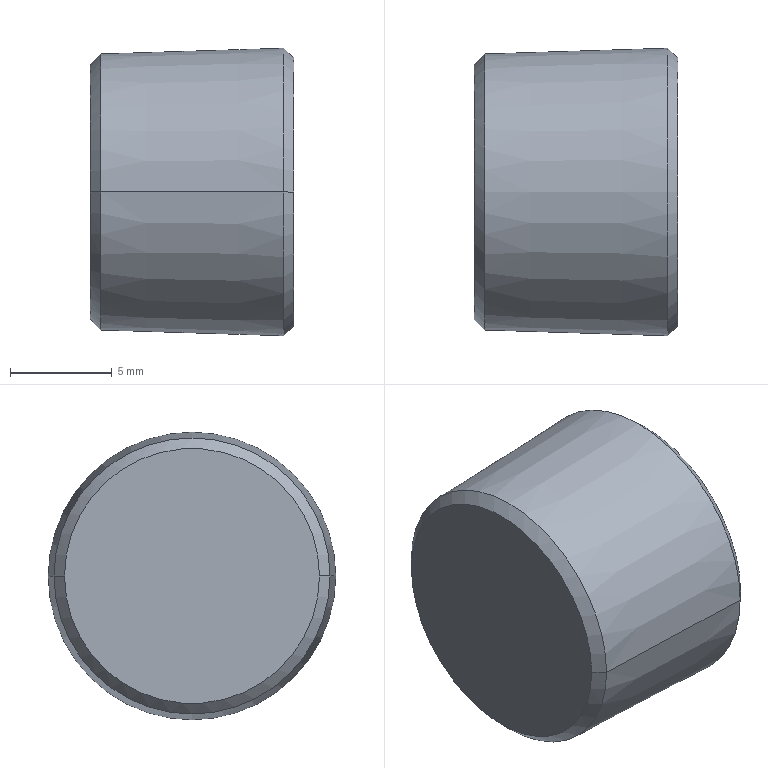Part | SolidWorks | features Chamfer 1, Cut 1, Revolution 1 | 1 solid | 15 faces | box 10 x 14.097 x 14.097 mm | volume 1197 mm3 | plane 9 | cone 6
STEP:
#1=CARTESIAN_POINT('',(0.,-6.25,0.));
#2=VERTEX_POINT('',#1);
#3=CARTESIAN_POINT('',(0.,6.25,0.));
#4=VERTEX_POINT('',#3);
#5=CARTESIAN_POINT('',(0.,0.,0.));
#6=DIRECTION('',(-1.,0.,0.));
#7=DIRECTION('',(0.,-1.,0.));
#8=AXIS2_PLACEMENT_3D('',#5,#6,#7);
#9=CIRCLE('',#8,6.25);
#10=EDGE_CURVE('',#2,#4,#9,.T.);
#11=ORIENTED_EDGE('',*,*,#10,.F.);
#12=CARTESIAN_POINT('',(0.5162,-6.766,0.));
#13=VERTEX_POINT('',#12);
#14=CARTESIAN_POINT('',(0.5162,-6.766,0.));
#15=DIRECTION('',(0.7071,-0.7071,0.));
#16=VECTOR('',#15,1000.);
#17=LINE('',#14,#16);
#18=EDGE_CURVE('',#2,#13,#17,.T.);
#19=ORIENTED_EDGE('',*,*,#18,.T.);
#20=CARTESIAN_POINT('',(0.5162,6.766,0.));
#21=VERTEX_POINT('',#20);
#22=CARTESIAN_POINT('',(0.5162,0.,0.));
#23=DIRECTION('',(1.,0.,0.));
#24=DIRECTION('',(0.,-1.,0.));
#25=AXIS2_PLACEMENT_3D('',#22,#23,#24);
#26=CIRCLE('',#25,6.766);
#27=EDGE_CURVE('',#21,#13,#26,.T.);
#28=ORIENTED_EDGE('',*,*,#27,.F.);
#29=CARTESIAN_POINT('',(0.5162,6.766,0.));
#30=DIRECTION('',(0.7071,0.7071,0.));
#31=VECTOR('',#30,1000.);
#32=LINE('',#29,#31);
#33=EDGE_CURVE('',#4,#21,#32,.T.);
#34=ORIENTED_EDGE('',*,*,#33,.F.);
#35=EDGE_LOOP('',(#11,#19,#28,#34));
#36=FACE_OUTER_BOUND('',#35,.T.);
#37=CARTESIAN_POINT('',(0.5162,0.,0.));
#38=DIRECTION('',(1.,0.,0.));
#39=DIRECTION('',(0.,1.,0.));
#40=AXIS2_PLACEMENT_3D('',#37,#38,#39);
#41=CONICAL_SURFACE('',#40,6.766,0.7854);
#42=ADVANCED_FACE('',(#36),#41,.T.);
#43=CARTESIAN_POINT('',(10.,6.579,0.));
#44=VERTEX_POINT('',#43);
#45=CARTESIAN_POINT('',(10.,-6.579,0.));
#46=VERTEX_POINT('',#45);
#47=CARTESIAN_POINT('',(10.,0.,0.));
#48=DIRECTION('',(1.,0.,0.));
#49=DIRECTION('',(0.,1.,0.));
#50=AXIS2_PLACEMENT_3D('',#47,#48,#49);
#51=CIRCLE('',#50,6.579);
#52=EDGE_CURVE('',#44,#46,#51,.T.);
#53=ORIENTED_EDGE('',*,*,#52,.F.);
#54=CARTESIAN_POINT('',(9.5,7.049,0.));
#55=VERTEX_POINT('',#54);
#56=CARTESIAN_POINT('',(10.,6.579,0.));
#57=DIRECTION('',(-0.729,0.6845,0.));
#58=VECTOR('',#57,1000.);
#59=LINE('',#56,#58);
#60=EDGE_CURVE('',#44,#55,#59,.T.);
#61=ORIENTED_EDGE('',*,*,#60,.T.);
#62=CARTESIAN_POINT('',(9.5,-7.049,0.));
#63=VERTEX_POINT('',#62);
#64=CARTESIAN_POINT('',(9.5,0.,0.));
#65=DIRECTION('',(-1.,0.,0.));
#66=DIRECTION('',(0.,-1.,0.));
#67=AXIS2_PLACEMENT_3D('',#64,#65,#66);
#68=CIRCLE('',#67,7.049);
#69=EDGE_CURVE('',#63,#55,#68,.T.);
#70=ORIENTED_EDGE('',*,*,#69,.F.);
#71=CARTESIAN_POINT('',(10.,-6.579,0.));
#72=DIRECTION('',(-0.729,-0.6845,0.));
#73=VECTOR('',#72,1000.);
#74=LINE('',#71,#73);
#75=EDGE_CURVE('',#46,#63,#74,.T.);
#76=ORIENTED_EDGE('',*,*,#75,.F.);
#77=EDGE_LOOP('',(#53,#61,#70,#76));
#78=FACE_OUTER_BOUND('',#77,.T.);
#79=CARTESIAN_POINT('',(10.,0.,0.));
#80=DIRECTION('',(-1.,0.,0.));
#81=DIRECTION('',(0.,-1.,0.));
#82=AXIS2_PLACEMENT_3D('',#79,#80,#81);
#83=CONICAL_SURFACE('',#82,6.579,0.754);
#84=ADVANCED_FACE('',(#78),#83,.T.);
#85=ORIENTED_EDGE('',*,*,#27,.T.);
#86=CARTESIAN_POINT('',(10.,-7.064,0.));
#87=DIRECTION('',(0.9995,-0.03141,0.));
#88=VECTOR('',#87,1000.);
#89=LINE('',#86,#88);
#90=EDGE_CURVE('',#13,#63,#89,.T.);
#91=ORIENTED_EDGE('',*,*,#90,.T.);
#92=ORIENTED_EDGE('',*,*,#69,.T.);
#93=CARTESIAN_POINT('',(10.,7.064,0.));
#94=DIRECTION('',(0.9995,0.03141,0.));
#95=VECTOR('',#94,1000.);
#96=LINE('',#93,#95);
#97=EDGE_CURVE('',#21,#55,#96,.T.);
#98=ORIENTED_EDGE('',*,*,#97,.F.);
#99=EDGE_LOOP('',(#85,#91,#92,#98));
#100=FACE_OUTER_BOUND('',#99,.T.);
#101=CARTESIAN_POINT('',(10.,0.,0.));
#102=DIRECTION('',(1.,0.,0.));
#103=DIRECTION('',(0.,1.,0.));
#104=AXIS2_PLACEMENT_3D('',#101,#102,#103);
#105=CONICAL_SURFACE('',#104,7.064,0.03142);
#106=ADVANCED_FACE('',(#100),#105,.T.);
#107=CARTESIAN_POINT('',(10.,0.,0.));
#108=DIRECTION('',(1.,0.,0.));
#109=DIRECTION('',(0.,1.,0.));
#110=AXIS2_PLACEMENT_3D('',#107,#108,#109);
#111=CIRCLE('',#110,6.579);
#112=EDGE_CURVE('',#46,#44,#111,.T.);
#113=ORIENTED_EDGE('',*,*,#112,.T.);
#114=ORIENTED_EDGE('',*,*,#52,.T.);
#115=EDGE_LOOP('',(#113,#114));
#116=FACE_OUTER_BOUND('',#115,.T.);
#117=CARTESIAN_POINT('',(10.,-4.1,2.367));
#118=VERTEX_POINT('',#117);
#119=CARTESIAN_POINT('',(10.,-4.1,-2.367));
#120=VERTEX_POINT('',#119);
#121=CARTESIAN_POINT('',(10.,-4.1,2.367));
#122=DIRECTION('',(0.,0.,-1.));
#123=VECTOR('',#122,1000.);
#124=LINE('',#121,#123);
#125=EDGE_CURVE('',#118,#120,#124,.T.);
#126=ORIENTED_EDGE('',*,*,#125,.F.);
#127=CARTESIAN_POINT('',(10.,0.,4.734));
#128=VERTEX_POINT('',#127);
#129=CARTESIAN_POINT('',(10.,0.,4.734));
#130=DIRECTION('',(0.,-0.866,-0.5));
#131=VECTOR('',#130,1000.);
#132=LINE('',#129,#131);
#133=EDGE_CURVE('',#128,#118,#132,.T.);
#134=ORIENTED_EDGE('',*,*,#133,.F.);
#135=CARTESIAN_POINT('',(10.,4.1,2.367));
#136=VERTEX_POINT('',#135);
#137=CARTESIAN_POINT('',(10.,4.1,2.367));
#138=DIRECTION('',(0.,-0.866,0.5));
#139=VECTOR('',#138,1000.);
#140=LINE('',#137,#139);
#141=EDGE_CURVE('',#136,#128,#140,.T.);
#142=ORIENTED_EDGE('',*,*,#141,.F.);
#143=CARTESIAN_POINT('',(10.,4.1,-2.367));
#144=VERTEX_POINT('',#143);
#145=CARTESIAN_POINT('',(10.,4.1,-2.367));
#146=DIRECTION('',(0.,0.,1.));
#147=VECTOR('',#146,1000.);
#148=LINE('',#145,#147);
#149=EDGE_CURVE('',#144,#136,#148,.T.);
#150=ORIENTED_EDGE('',*,*,#149,.F.);
#151=CARTESIAN_POINT('',(10.,0.,-4.734));
#152=VERTEX_POINT('',#151);
#153=CARTESIAN_POINT('',(10.,0.,-4.734));
#154=DIRECTION('',(0.,0.866,0.5));
#155=VECTOR('',#154,1000.);
#156=LINE('',#153,#155);
#157=EDGE_CURVE('',#152,#144,#156,.T.);
#158=ORIENTED_EDGE('',*,*,#157,.F.);
#159=CARTESIAN_POINT('',(10.,-4.1,-2.367));
#160=DIRECTION('',(0.,0.866,-0.5));
#161=VECTOR('',#160,1000.);
#162=LINE('',#159,#161);
#163=EDGE_CURVE('',#120,#152,#162,.T.);
#164=ORIENTED_EDGE('',*,*,#163,.F.);
#165=EDGE_LOOP('',(#126,#134,#142,#150,#158,#164));
#166=FACE_BOUND('',#165,.T.);
#167=CARTESIAN_POINT('',(10.,7.064,0.));
#168=DIRECTION('',(1.,0.,0.));
#169=DIRECTION('',(0.,1.,0.));
#170=AXIS2_PLACEMENT_3D('',#167,#168,#169);
#171=PLANE('',#170);
#172=ADVANCED_FACE('',(#116,#166),#171,.T.);
#173=ORIENTED_EDGE('',*,*,#90,.F.);
#174=CARTESIAN_POINT('',(0.5162,0.,0.));
#175=DIRECTION('',(1.,0.,0.));
#176=DIRECTION('',(0.,-1.,0.));
#177=AXIS2_PLACEMENT_3D('',#174,#175,#176);
#178=CIRCLE('',#177,6.766);
#179=EDGE_CURVE('',#13,#21,#178,.T.);
#180=ORIENTED_EDGE('',*,*,#179,.T.);
#181=ORIENTED_EDGE('',*,*,#97,.T.);
#182=CARTESIAN_POINT('',(9.5,0.,0.));
#183=DIRECTION('',(-1.,0.,0.));
#184=DIRECTION('',(0.,-1.,0.));
#185=AXIS2_PLACEMENT_3D('',#182,#183,#184);
#186=CIRCLE('',#185,7.049);
#187=EDGE_CURVE('',#55,#63,#186,.T.);
#188=ORIENTED_EDGE('',*,*,#187,.T.);
#189=EDGE_LOOP('',(#173,#180,#181,#188));
#190=FACE_OUTER_BOUND('',#189,.T.);
#191=CARTESIAN_POINT('',(10.,0.,0.));
#192=DIRECTION('',(1.,0.,0.));
#193=DIRECTION('',(0.,1.,0.));
#194=AXIS2_PLACEMENT_3D('',#191,#192,#193);
#195=CONICAL_SURFACE('',#194,7.064,0.03142);
#196=ADVANCED_FACE('',(#190),#195,.T.);
#197=CARTESIAN_POINT('',(0.,0.,0.));
#198=DIRECTION('',(-1.,0.,0.));
#199=DIRECTION('',(0.,-1.,0.));
#200=AXIS2_PLACEMENT_3D('',#197,#198,#199);
#201=CIRCLE('',#200,6.25);
#202=EDGE_CURVE('',#4,#2,#201,.T.);
#203=ORIENTED_EDGE('',*,*,#202,.T.);
#204=ORIENTED_EDGE('',*,*,#10,.T.);
#205=EDGE_LOOP('',(#203,#204));
#206=FACE_OUTER_BOUND('',#205,.T.);
#207=CARTESIAN_POINT('',(0.,0.,0.));
#208=DIRECTION('',(-1.,0.,0.));
#209=DIRECTION('',(0.,-1.,0.));
#210=AXIS2_PLACEMENT_3D('',#207,#208,#209);
#211=PLANE('',#210);
#212=ADVANCED_FACE('',(#206),#211,.T.);
#213=ORIENTED_EDGE('',*,*,#125,.T.);
#214=CARTESIAN_POINT('',(5.,-4.1,-2.367));
#215=VERTEX_POINT('',#214);
#216=CARTESIAN_POINT('',(5.,-4.1,-2.367));
#217=DIRECTION('',(1.,0.,0.));
#218=VECTOR('',#217,1000.);
#219=LINE('',#216,#218);
#220=EDGE_CURVE('',#215,#120,#219,.T.);
#221=ORIENTED_EDGE('',*,*,#220,.F.);
#222=CARTESIAN_POINT('',(5.,-4.1,2.367));
#223=VERTEX_POINT('',#222);
#224=CARTESIAN_POINT('',(5.,-4.1,2.367));
#225=DIRECTION('',(0.,0.,-1.));
#226=VECTOR('',#225,1000.);
#227=LINE('',#224,#226);
#228=EDGE_CURVE('',#223,#215,#227,.T.);
#229=ORIENTED_EDGE('',*,*,#228,.F.);
#230=CARTESIAN_POINT('',(5.,-4.1,2.367));
#231=DIRECTION('',(1.,0.,0.));
#232=VECTOR('',#231,1000.);
#233=LINE('',#230,#232);
#234=EDGE_CURVE('',#223,#118,#233,.T.);
#235=ORIENTED_EDGE('',*,*,#234,.T.);
#236=EDGE_LOOP('',(#213,#221,#229,#235));
#237=FACE_OUTER_BOUND('',#236,.T.);
#238=CARTESIAN_POINT('',(5.,-4.1,2.367));
#239=DIRECTION('',(0.,-1.,0.));
#240=DIRECTION('',(0.,0.,-1.));
#241=AXIS2_PLACEMENT_3D('',#238,#239,#240);
#242=PLANE('',#241);
#243=ADVANCED_FACE('',(#237),#242,.F.);
#244=ORIENTED_EDGE('',*,*,#133,.T.);
#245=ORIENTED_EDGE('',*,*,#234,.F.);
#246=CARTESIAN_POINT('',(5.,0.,4.734));
#247=VERTEX_POINT('',#246);
#248=CARTESIAN_POINT('',(5.,0.,4.734));
#249=DIRECTION('',(0.,-0.866,-0.5));
#250=VECTOR('',#249,1000.);
#251=LINE('',#248,#250);
#252=EDGE_CURVE('',#247,#223,#251,.T.);
#253=ORIENTED_EDGE('',*,*,#252,.F.);
#254=CARTESIAN_POINT('',(5.,0.,4.734));
#255=DIRECTION('',(1.,0.,0.));
#256=VECTOR('',#255,1000.);
#257=LINE('',#254,#256);
#258=EDGE_CURVE('',#247,#128,#257,.T.);
#259=ORIENTED_EDGE('',*,*,#258,.T.);
#260=EDGE_LOOP('',(#244,#245,#253,#259));
#261=FACE_OUTER_BOUND('',#260,.T.);
#262=CARTESIAN_POINT('',(5.,0.,4.734));
#263=DIRECTION('',(0.,-0.5,0.866));
#264=DIRECTION('',(0.,-0.866,-0.5));
#265=AXIS2_PLACEMENT_3D('',#262,#263,#264);
#266=PLANE('',#265);
#267=ADVANCED_FACE('',(#261),#266,.F.);
#268=ORIENTED_EDGE('',*,*,#141,.T.);
#269=ORIENTED_EDGE('',*,*,#258,.F.);
#270=CARTESIAN_POINT('',(5.,4.1,2.367));
#271=VERTEX_POINT('',#270);
#272=CARTESIAN_POINT('',(5.,4.1,2.367));
#273=DIRECTION('',(0.,-0.866,0.5));
#274=VECTOR('',#273,1000.);
#275=LINE('',#272,#274);
#276=EDGE_CURVE('',#271,#247,#275,.T.);
#277=ORIENTED_EDGE('',*,*,#276,.F.);
#278=CARTESIAN_POINT('',(5.,4.1,2.367));
#279=DIRECTION('',(1.,0.,0.));
#280=VECTOR('',#279,1000.);
#281=LINE('',#278,#280);
#282=EDGE_CURVE('',#271,#136,#281,.T.);
#283=ORIENTED_EDGE('',*,*,#282,.T.);
#284=EDGE_LOOP('',(#268,#269,#277,#283));
#285=FACE_OUTER_BOUND('',#284,.T.);
#286=CARTESIAN_POINT('',(5.,4.1,2.367));
#287=DIRECTION('',(0.,0.5,0.866));
#288=DIRECTION('',(0.,-0.866,0.5));
#289=AXIS2_PLACEMENT_3D('',#286,#287,#288);
#290=PLANE('',#289);
#291=ADVANCED_FACE('',(#285),#290,.F.);
#292=ORIENTED_EDGE('',*,*,#149,.T.);
#293=ORIENTED_EDGE('',*,*,#282,.F.);
#294=CARTESIAN_POINT('',(5.,4.1,-2.367));
#295=VERTEX_POINT('',#294);
#296=CARTESIAN_POINT('',(5.,4.1,-2.367));
#297=DIRECTION('',(0.,0.,1.));
#298=VECTOR('',#297,1000.);
#299=LINE('',#296,#298);
#300=EDGE_CURVE('',#295,#271,#299,.T.);
#301=ORIENTED_EDGE('',*,*,#300,.F.);
#302=CARTESIAN_POINT('',(5.,4.1,-2.367));
#303=DIRECTION('',(1.,0.,0.));
#304=VECTOR('',#303,1000.);
#305=LINE('',#302,#304);
#306=EDGE_CURVE('',#295,#144,#305,.T.);
#307=ORIENTED_EDGE('',*,*,#306,.T.);
#308=EDGE_LOOP('',(#292,#293,#301,#307));
#309=FACE_OUTER_BOUND('',#308,.T.);
#310=CARTESIAN_POINT('',(5.,4.1,-2.367));
#311=DIRECTION('',(0.,1.,0.));
#312=DIRECTION('',(0.,0.,1.));
#313=AXIS2_PLACEMENT_3D('',#310,#311,#312);
#314=PLANE('',#313);
#315=ADVANCED_FACE('',(#309),#314,.F.);
#316=ORIENTED_EDGE('',*,*,#157,.T.);
#317=ORIENTED_EDGE('',*,*,#306,.F.);
#318=CARTESIAN_POINT('',(5.,0.,-4.734));
#319=VERTEX_POINT('',#318);
#320=CARTESIAN_POINT('',(5.,0.,-4.734));
#321=DIRECTION('',(0.,0.866,0.5));
#322=VECTOR('',#321,1000.);
#323=LINE('',#320,#322);
#324=EDGE_CURVE('',#319,#295,#323,.T.);
#325=ORIENTED_EDGE('',*,*,#324,.F.);
#326=CARTESIAN_POINT('',(5.,0.,-4.734));
#327=DIRECTION('',(1.,0.,0.));
#328=VECTOR('',#327,1000.);
#329=LINE('',#326,#328);
#330=EDGE_CURVE('',#319,#152,#329,.T.);
#331=ORIENTED_EDGE('',*,*,#330,.T.);
#332=EDGE_LOOP('',(#316,#317,#325,#331));
#333=FACE_OUTER_BOUND('',#332,.T.);
#334=CARTESIAN_POINT('',(5.,0.,-4.734));
#335=DIRECTION('',(0.,0.5,-0.866));
#336=DIRECTION('',(0.,0.866,0.5));
#337=AXIS2_PLACEMENT_3D('',#334,#335,#336);
#338=PLANE('',#337);
#339=ADVANCED_FACE('',(#333),#338,.F.);
#340=ORIENTED_EDGE('',*,*,#163,.T.);
#341=ORIENTED_EDGE('',*,*,#330,.F.);
#342=CARTESIAN_POINT('',(5.,-4.1,-2.367));
#343=DIRECTION('',(0.,0.866,-0.5));
#344=VECTOR('',#343,1000.);
#345=LINE('',#342,#344);
#346=EDGE_CURVE('',#215,#319,#345,.T.);
#347=ORIENTED_EDGE('',*,*,#346,.F.);
#348=ORIENTED_EDGE('',*,*,#220,.T.);
#349=EDGE_LOOP('',(#340,#341,#347,#348));
#350=FACE_OUTER_BOUND('',#349,.T.);
#351=CARTESIAN_POINT('',(5.,-4.1,-2.367));
#352=DIRECTION('',(0.,-0.5,-0.866));
#353=DIRECTION('',(0.,0.866,-0.5));
#354=AXIS2_PLACEMENT_3D('',#351,#352,#353);
#355=PLANE('',#354);
#356=ADVANCED_FACE('',(#350),#355,.F.);
#357=ORIENTED_EDGE('',*,*,#228,.T.);
#358=ORIENTED_EDGE('',*,*,#346,.T.);
#359=ORIENTED_EDGE('',*,*,#324,.T.);
#360=ORIENTED_EDGE('',*,*,#300,.T.);
#361=ORIENTED_EDGE('',*,*,#276,.T.);
#362=ORIENTED_EDGE('',*,*,#252,.T.);
#363=EDGE_LOOP('',(#357,#358,#359,#360,#361,#362));
#364=FACE_OUTER_BOUND('',#363,.T.);
#365=CARTESIAN_POINT('',(5.,-4.1,2.367));
#366=DIRECTION('',(-1.,0.,0.));
#367=DIRECTION('',(0.,0.,1.));
#368=AXIS2_PLACEMENT_3D('',#365,#366,#367);
#369=PLANE('',#368);
#370=ADVANCED_FACE('',(#364),#369,.F.);
#371=ORIENTED_EDGE('',*,*,#60,.F.);
#372=ORIENTED_EDGE('',*,*,#112,.F.);
#373=ORIENTED_EDGE('',*,*,#75,.T.);
#374=ORIENTED_EDGE('',*,*,#187,.F.);
#375=EDGE_LOOP('',(#371,#372,#373,#374));
#376=FACE_OUTER_BOUND('',#375,.T.);
#377=CARTESIAN_POINT('',(10.,0.,0.));
#378=DIRECTION('',(-1.,0.,0.));
#379=DIRECTION('',(0.,-1.,0.));
#380=AXIS2_PLACEMENT_3D('',#377,#378,#379);
#381=CONICAL_SURFACE('',#380,6.579,0.754);
#382=ADVANCED_FACE('',(#376),#381,.T.);
#383=ORIENTED_EDGE('',*,*,#18,.F.);
#384=ORIENTED_EDGE('',*,*,#202,.F.);
#385=ORIENTED_EDGE('',*,*,#33,.T.);
#386=ORIENTED_EDGE('',*,*,#179,.F.);
#387=EDGE_LOOP('',(#383,#384,#385,#386));
#388=FACE_OUTER_BOUND('',#387,.T.);
#389=CARTESIAN_POINT('',(0.5162,0.,0.));
#390=DIRECTION('',(1.,0.,0.));
#391=DIRECTION('',(0.,1.,0.));
#392=AXIS2_PLACEMENT_3D('',#389,#390,#391);
#393=CONICAL_SURFACE('',#392,6.766,0.7854);
#394=ADVANCED_FACE('',(#388),#393,.T.);
#395=CLOSED_SHELL('',(#42,#84,#106,#172,#196,#212,#243,#267,#291,#315,#339,#356,#370,#382,#394));
#396=MANIFOLD_SOLID_BREP('',#395);
#397=CARTESIAN_POINT('',(0.,0.,0.));
#398=DIRECTION('',(0.,0.,1.));
#399=DIRECTION('',(1.,0.,0.));
#400=AXIS2_PLACEMENT_3D('',#397,#398,#399);
#401=(LENGTH_UNIT()NAMED_UNIT(*)SI_UNIT(.MILLI.,.METRE.));
#402=UNCERTAINTY_MEASURE_WITH_UNIT(LENGTH_MEASURE(0.00001),#401,'','');
#403=(NAMED_UNIT(*)PLANE_ANGLE_UNIT()SI_UNIT($,.RADIAN.));
#404=(NAMED_UNIT(*)SI_UNIT($,.STERADIAN.)SOLID_ANGLE_UNIT());
#405=(GEOMETRIC_REPRESENTATION_CONTEXT(3)GLOBAL_UNCERTAINTY_ASSIGNED_CONTEXT((#402))GLOBAL_UNIT_ASSIGNED_CONTEXT((#401,#403,#404))REPRESENTATION_CONTEXT('',''));
#406=ADVANCED_BREP_SHAPE_REPRESENTATION('',(#396,#400),#405);